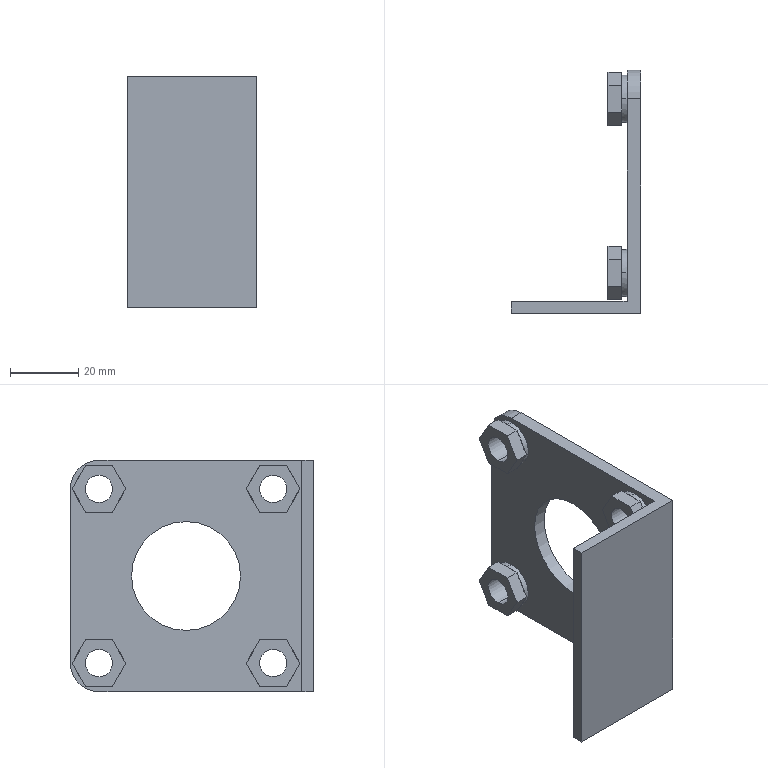Part | SolidWorks | features BaseBody 1 | 1 solid | 104 faces | box 38 x 71.5 x 68 mm | volume 25809 mm3 | plane 84 | cylinder 20 | commonest cylinder face diameters 8 x8 13.92 x8 16.8 x2 32 x2